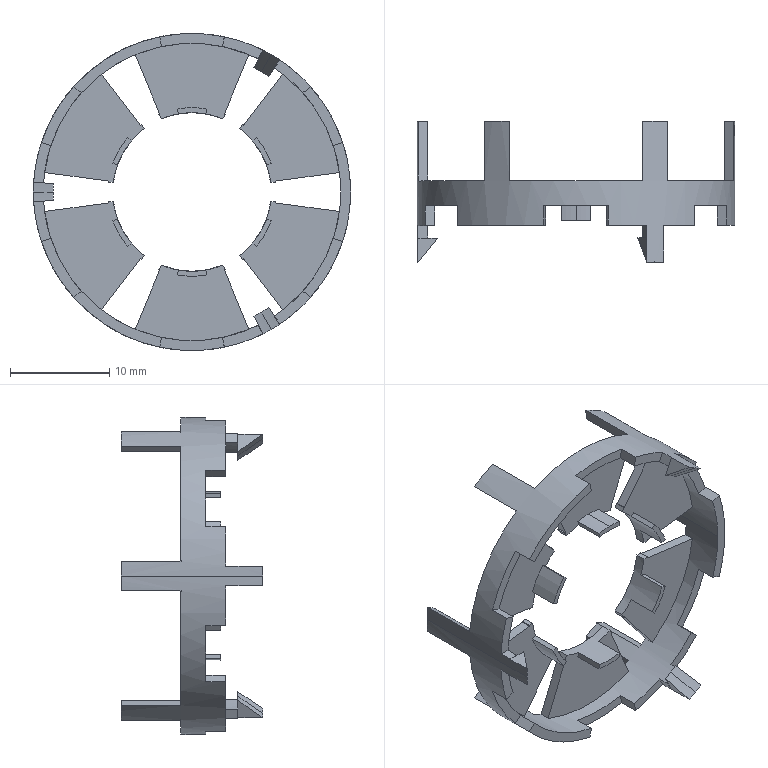Part | SolidWorks | features BaseBody 1 | 1 solid | 156 faces | box 32.01 x 14.281 x 32 mm | volume 874.407 mm3 | plane 120 | cylinder 30 | cone 6 | commonest cylinder face diameters 17 x19 16 x7 30 x2 32 x2